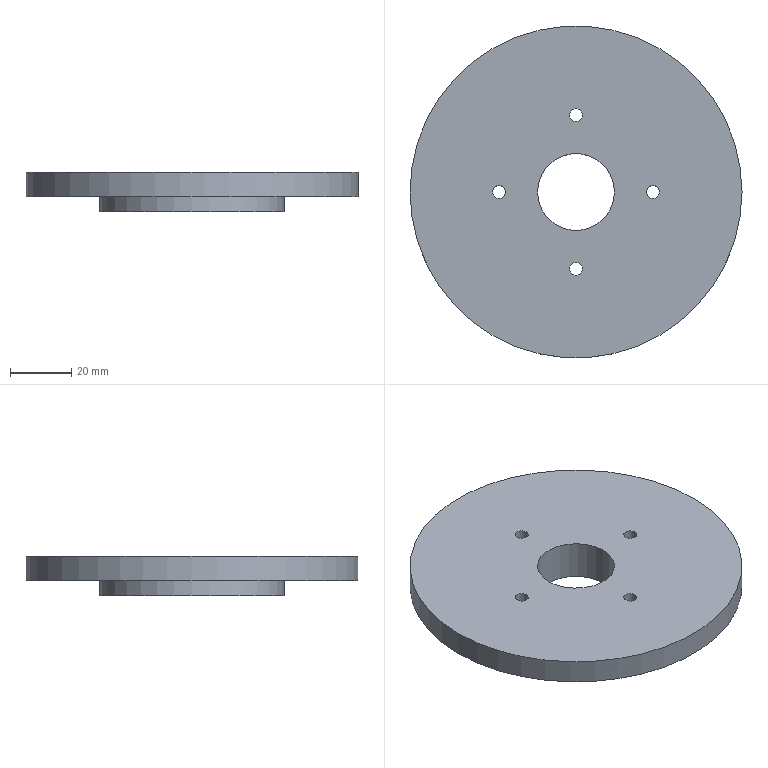CAM job | NX | 3-axis milling, drilling | part box 108 x 108 x 13 mm | stock box 108 x 108 x 13 mm
Tools:
number,name,description,diameter,corner_radius,flute_length,length,flutes
1,ZXZ,Milling Tool-5 Parameters,6.0,0.0,50.0,75.0,2
7,D6A45,Milling Tool-5 Parameters,6.0,0.0,3.0,3.0,2
2,4.2ZT,Drilling Tool,4.2,0.0,35.0,50.0,2
Operations:
program,operation,operation_type,tool,method,geometry_group,spindle_rpm,surface_speed,feed_per_tooth,feed_cut,feed_plunge,cut_length_mm,path_length_mm,cut_time_min,machine_time_min
1,DRILLING,Operation,ZXZ,METHOD,A,3000.0,56.0,0.0333,200.0,0.0,16.0,207.447,0.08,0.0991
1,DRILLING_COPY,Operation,4.2ZT,METHOD,A,2000.0,26.0,0.0275,110.0,0.0,75.047,325.542,0.6822,0.7073
1,ZLEVEL_PROFILE_1_COPY_1,ZLevelMilling,D6A45,METHOD,A,7500.0,141.0,0.0667,1000.0,100.0,52.084,412.897,0.0521,0.0882